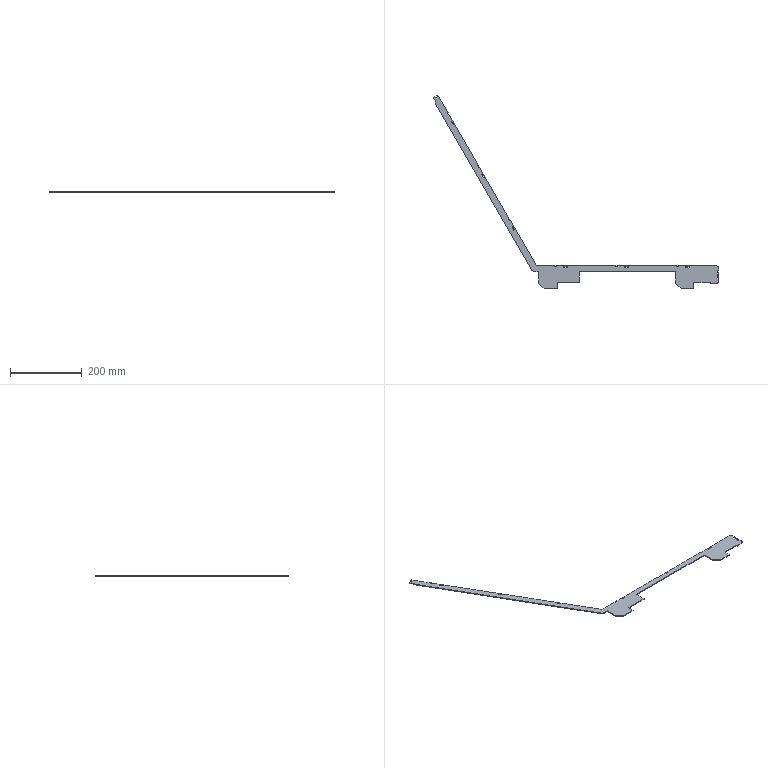Part | STEP file | zh005-1 | 1 solid | 87 faces | box 796.98 x 541.285 x 2 mm | volume 53222 mm3 | plane 84 | cylinder 3 | commonest cylinder face diameters 16 x2 20 x1